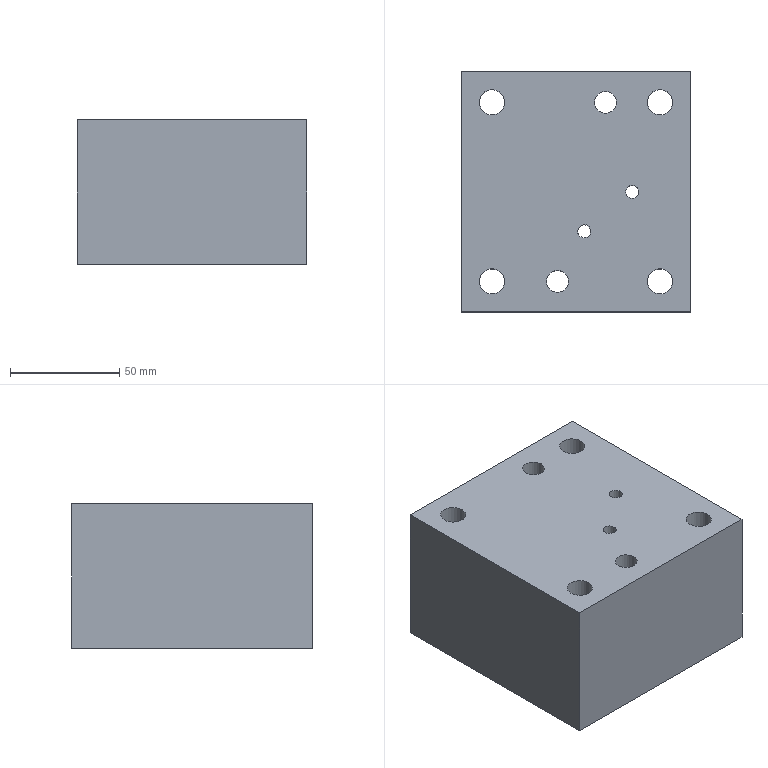Part | NX | features solid 2 | 1 solid | 32 faces | box 105 x 110 x 66.13 mm | volume 695141 mm3 | cylinder 16 | plane 12 | cone 4 | commonest cylinder face diameters 11.507 x4 18.008 x4 6 x2 8.5 x2 10 x2 12.505 x2
STEP:
#1=CARTESIAN_POINT('',(751.736,37.878,115.));
#2=VERTEX_POINT('',#1);
#3=CARTESIAN_POINT('',(751.736,28.874,115.));
#4=DIRECTION('',(0.000000053,-0.000000517,1.));
#5=DIRECTION('',(0.,1.,0.000000517));
#6=AXIS2_PLACEMENT_3D('',#3,#4,#5);
#7=CIRCLE('',#6,9.004);
#8=EDGE_CURVE('',#2,#2,#7,.T.);
#9=ORIENTED_EDGE('',*,*,#8,.T.);
#10=EDGE_LOOP('',(#9));
#11=FACE_BOUND('',#10,.T.);
#12=CARTESIAN_POINT('',(674.736,37.878,115.));
#13=VERTEX_POINT('',#12);
#14=CARTESIAN_POINT('',(674.736,28.874,115.));
#15=DIRECTION('',(0.000000053,-0.000000517,1.));
#16=DIRECTION('',(0.,1.,0.000000517));
#17=AXIS2_PLACEMENT_3D('',#14,#15,#16);
#18=CIRCLE('',#17,9.004);
#19=EDGE_CURVE('',#13,#13,#18,.T.);
#20=ORIENTED_EDGE('',*,*,#19,.T.);
#21=EDGE_LOOP('',(#20));
#22=FACE_BOUND('',#21,.T.);
#23=CARTESIAN_POINT('',(660.736,124.874,115.));
#24=VERTEX_POINT('',#23);
#25=CARTESIAN_POINT('',(660.736,14.874,115.));
#26=VERTEX_POINT('',#25);
#27=CARTESIAN_POINT('',(660.736,69.874,115.));
#28=DIRECTION('',(0.,1.,0.000000517));
#29=VECTOR('',#28,1000.);
#30=LINE('',#27,#29);
#31=EDGE_CURVE('',#24,#26,#30,.F.);
#32=ORIENTED_EDGE('',*,*,#31,.F.);
#33=CARTESIAN_POINT('',(765.736,124.874,115.));
#34=VERTEX_POINT('',#33);
#35=CARTESIAN_POINT('',(713.236,124.874,115.));
#36=DIRECTION('',(1.,0.,-0.000000053));
#37=VECTOR('',#36,1000.);
#38=LINE('',#35,#37);
#39=EDGE_CURVE('',#34,#24,#38,.F.);
#40=ORIENTED_EDGE('',*,*,#39,.F.);
#41=CARTESIAN_POINT('',(765.736,14.874,115.));
#42=VERTEX_POINT('',#41);
#43=CARTESIAN_POINT('',(765.736,69.874,115.));
#44=DIRECTION('',(0.,-1.,-0.000000517));
#45=VECTOR('',#44,1000.);
#46=LINE('',#43,#45);
#47=EDGE_CURVE('',#42,#34,#46,.F.);
#48=ORIENTED_EDGE('',*,*,#47,.F.);
#49=CARTESIAN_POINT('',(713.236,14.874,115.));
#50=DIRECTION('',(-1.,0.,0.000000053));
#51=VECTOR('',#50,1000.);
#52=LINE('',#49,#51);
#53=EDGE_CURVE('',#26,#42,#52,.F.);
#54=ORIENTED_EDGE('',*,*,#53,.F.);
#55=EDGE_LOOP('',(#32,#40,#48,#54));
#56=FACE_BOUND('',#55,.T.);
#57=CARTESIAN_POINT('',(751.736,119.878,115.));
#58=VERTEX_POINT('',#57);
#59=CARTESIAN_POINT('',(751.736,110.874,115.));
#60=DIRECTION('',(0.000000053,-0.000000517,1.));
#61=DIRECTION('',(0.,1.,0.000000517));
#62=AXIS2_PLACEMENT_3D('',#59,#60,#61);
#63=CIRCLE('',#62,9.004);
#64=EDGE_CURVE('',#58,#58,#63,.T.);
#65=ORIENTED_EDGE('',*,*,#64,.T.);
#66=EDGE_LOOP('',(#65));
#67=FACE_BOUND('',#66,.T.);
#68=CARTESIAN_POINT('',(674.736,119.878,115.));
#69=VERTEX_POINT('',#68);
#70=CARTESIAN_POINT('',(674.736,110.874,115.));
#71=DIRECTION('',(0.000000053,-0.000000517,1.));
#72=DIRECTION('',(0.,1.,0.000000517));
#73=AXIS2_PLACEMENT_3D('',#70,#71,#72);
#74=CIRCLE('',#73,9.004);
#75=EDGE_CURVE('',#69,#69,#74,.T.);
#76=ORIENTED_EDGE('',*,*,#75,.T.);
#77=EDGE_LOOP('',(#76));
#78=FACE_BOUND('',#77,.T.);
#79=CARTESIAN_POINT('',(726.736,117.126,115.));
#80=VERTEX_POINT('',#79);
#81=CARTESIAN_POINT('',(726.736,110.874,115.));
#82=DIRECTION('',(0.000000053,-0.000000517,1.));
#83=DIRECTION('',(0.,1.,0.000000517));
#84=AXIS2_PLACEMENT_3D('',#81,#82,#83);
#85=CIRCLE('',#84,6.253);
#86=EDGE_CURVE('',#80,#80,#85,.F.);
#87=ORIENTED_EDGE('',*,*,#86,.F.);
#88=EDGE_LOOP('',(#87));
#89=FACE_BOUND('',#88,.T.);
#90=CARTESIAN_POINT('',(704.736,35.126,115.));
#91=VERTEX_POINT('',#90);
#92=CARTESIAN_POINT('',(704.736,28.874,115.));
#93=DIRECTION('',(0.000000053,-0.000000517,1.));
#94=DIRECTION('',(0.,1.,0.000000517));
#95=AXIS2_PLACEMENT_3D('',#92,#93,#94);
#96=CIRCLE('',#95,6.253);
#97=EDGE_CURVE('',#91,#91,#96,.F.);
#98=ORIENTED_EDGE('',*,*,#97,.F.);
#99=EDGE_LOOP('',(#98));
#100=FACE_BOUND('',#99,.T.);
#101=CARTESIAN_POINT('',(729.986,79.874,115.));
#102=VERTEX_POINT('',#101);
#103=CARTESIAN_POINT('',(729.986,84.874,115.));
#104=DIRECTION('',(0.000000053,-0.000000517,1.));
#105=DIRECTION('',(0.,-1.,-0.000000517));
#106=AXIS2_PLACEMENT_3D('',#103,#104,#105);
#107=CIRCLE('',#106,5.);
#108=EDGE_CURVE('',#102,#102,#107,.T.);
#109=ORIENTED_EDGE('',*,*,#108,.T.);
#110=EDGE_LOOP('',(#109));
#111=FACE_BOUND('',#110,.T.);
#112=CARTESIAN_POINT('',(729.986,49.874,115.));
#113=VERTEX_POINT('',#112);
#114=CARTESIAN_POINT('',(729.986,54.874,115.));
#115=DIRECTION('',(0.000000053,-0.000000517,1.));
#116=DIRECTION('',(0.,-1.,-0.000000517));
#117=AXIS2_PLACEMENT_3D('',#114,#115,#116);
#118=CIRCLE('',#117,5.);
#119=EDGE_CURVE('',#113,#113,#118,.T.);
#120=ORIENTED_EDGE('',*,*,#119,.T.);
#121=EDGE_LOOP('',(#120));
#122=FACE_BOUND('',#121,.T.);
#123=CARTESIAN_POINT('',(716.986,48.874,115.));
#124=VERTEX_POINT('',#123);
#125=CARTESIAN_POINT('',(716.986,51.874,115.));
#126=DIRECTION('',(0.000000053,-0.000000517,1.));
#127=DIRECTION('',(0.,-1.,-0.000000517));
#128=AXIS2_PLACEMENT_3D('',#125,#126,#127);
#129=CIRCLE('',#128,3.);
#130=EDGE_CURVE('',#124,#124,#129,.F.);
#131=ORIENTED_EDGE('',*,*,#130,.F.);
#132=EDGE_LOOP('',(#131));
#133=FACE_BOUND('',#132,.T.);
#134=CARTESIAN_POINT('',(738.986,66.874,115.));
#135=VERTEX_POINT('',#134);
#136=CARTESIAN_POINT('',(738.986,69.874,115.));
#137=DIRECTION('',(0.000000053,-0.000000517,1.));
#138=DIRECTION('',(0.,-1.,-0.000000517));
#139=AXIS2_PLACEMENT_3D('',#136,#137,#138);
#140=CIRCLE('',#139,3.);
#141=EDGE_CURVE('',#135,#135,#140,.T.);
#142=ORIENTED_EDGE('',*,*,#141,.T.);
#143=EDGE_LOOP('',(#142));
#144=FACE_BOUND('',#143,.T.);
#145=CARTESIAN_POINT('',(735.986,94.874,115.));
#146=DIRECTION('',(0.000000053,-0.000000517,1.));
#147=DIRECTION('',(0.,1.,0.000000517));
#148=AXIS2_PLACEMENT_3D('',#145,#146,#147);
#149=PLANE('',#148);
#150=ADVANCED_FACE('',(#11,#22,#56,#67,#78,#89,#100,#111,#122,#133,#144),#149,.F.);
#151=CARTESIAN_POINT('',(660.736,124.874,181.13));
#152=VERTEX_POINT('',#151);
#153=CARTESIAN_POINT('',(765.736,124.874,181.13));
#154=VERTEX_POINT('',#153);
#155=CARTESIAN_POINT('',(713.236,124.874,181.13));
#156=DIRECTION('',(1.,0.,0.));
#157=VECTOR('',#156,1000.);
#158=LINE('',#155,#157);
#159=EDGE_CURVE('',#152,#154,#158,.T.);
#160=ORIENTED_EDGE('',*,*,#159,.F.);
#161=CARTESIAN_POINT('',(660.736,14.874,181.13));
#162=VERTEX_POINT('',#161);
#163=CARTESIAN_POINT('',(660.736,69.874,181.13));
#164=DIRECTION('',(0.,1.,0.));
#165=VECTOR('',#164,1000.);
#166=LINE('',#163,#165);
#167=EDGE_CURVE('',#162,#152,#166,.T.);
#168=ORIENTED_EDGE('',*,*,#167,.F.);
#169=CARTESIAN_POINT('',(765.736,14.874,181.13));
#170=VERTEX_POINT('',#169);
#171=CARTESIAN_POINT('',(713.236,14.874,181.13));
#172=DIRECTION('',(-1.,0.,0.));
#173=VECTOR('',#172,1000.);
#174=LINE('',#171,#173);
#175=EDGE_CURVE('',#170,#162,#174,.T.);
#176=ORIENTED_EDGE('',*,*,#175,.F.);
#177=CARTESIAN_POINT('',(765.736,69.874,181.13));
#178=DIRECTION('',(0.,-1.,0.));
#179=VECTOR('',#178,1000.);
#180=LINE('',#177,#179);
#181=EDGE_CURVE('',#154,#170,#180,.T.);
#182=ORIENTED_EDGE('',*,*,#181,.F.);
#183=EDGE_LOOP('',(#160,#168,#176,#182));
#184=FACE_BOUND('',#183,.T.);
#185=CARTESIAN_POINT('',(745.983,110.874,181.13));
#186=VERTEX_POINT('',#185);
#187=CARTESIAN_POINT('',(751.736,110.874,181.13));
#188=DIRECTION('',(0.,0.,1.));
#189=DIRECTION('',(-1.,0.,0.));
#190=AXIS2_PLACEMENT_3D('',#187,#188,#189);
#191=CIRCLE('',#190,5.753);
#192=EDGE_CURVE('',#186,#186,#191,.T.);
#193=ORIENTED_EDGE('',*,*,#192,.F.);
#194=EDGE_LOOP('',(#193));
#195=FACE_BOUND('',#194,.T.);
#196=CARTESIAN_POINT('',(668.983,28.874,181.13));
#197=VERTEX_POINT('',#196);
#198=CARTESIAN_POINT('',(674.736,28.874,181.13));
#199=DIRECTION('',(0.,0.,1.));
#200=DIRECTION('',(-1.,0.,0.));
#201=AXIS2_PLACEMENT_3D('',#198,#199,#200);
#202=CIRCLE('',#201,5.753);
#203=EDGE_CURVE('',#197,#197,#202,.T.);
#204=ORIENTED_EDGE('',*,*,#203,.F.);
#205=EDGE_LOOP('',(#204));
#206=FACE_BOUND('',#205,.T.);
#207=CARTESIAN_POINT('',(668.983,110.874,181.13));
#208=VERTEX_POINT('',#207);
#209=CARTESIAN_POINT('',(674.736,110.874,181.13));
#210=DIRECTION('',(0.,0.,1.));
#211=DIRECTION('',(-1.,0.,0.));
#212=AXIS2_PLACEMENT_3D('',#209,#210,#211);
#213=CIRCLE('',#212,5.753);
#214=EDGE_CURVE('',#208,#208,#213,.T.);
#215=ORIENTED_EDGE('',*,*,#214,.F.);
#216=EDGE_LOOP('',(#215));
#217=FACE_BOUND('',#216,.T.);
#218=CARTESIAN_POINT('',(745.983,28.874,181.13));
#219=VERTEX_POINT('',#218);
#220=CARTESIAN_POINT('',(751.736,28.874,181.13));
#221=DIRECTION('',(0.,0.,1.));
#222=DIRECTION('',(-1.,0.,0.));
#223=AXIS2_PLACEMENT_3D('',#220,#221,#222);
#224=CIRCLE('',#223,5.753);
#225=EDGE_CURVE('',#219,#219,#224,.T.);
#226=ORIENTED_EDGE('',*,*,#225,.F.);
#227=EDGE_LOOP('',(#226));
#228=FACE_BOUND('',#227,.T.);
#229=CARTESIAN_POINT('',(721.736,110.874,181.13));
#230=VERTEX_POINT('',#229);
#231=CARTESIAN_POINT('',(726.736,110.874,181.13));
#232=DIRECTION('',(0.,0.,1.));
#233=DIRECTION('',(-1.,0.,0.));
#234=AXIS2_PLACEMENT_3D('',#231,#232,#233);
#235=CIRCLE('',#234,5.);
#236=EDGE_CURVE('',#230,#230,#235,.T.);
#237=ORIENTED_EDGE('',*,*,#236,.F.);
#238=EDGE_LOOP('',(#237));
#239=FACE_BOUND('',#238,.T.);
#240=CARTESIAN_POINT('',(699.736,28.874,181.13));
#241=VERTEX_POINT('',#240);
#242=CARTESIAN_POINT('',(704.736,28.874,181.13));
#243=DIRECTION('',(0.,0.,1.));
#244=DIRECTION('',(-1.,0.,0.));
#245=AXIS2_PLACEMENT_3D('',#242,#243,#244);
#246=CIRCLE('',#245,5.);
#247=EDGE_CURVE('',#241,#241,#246,.T.);
#248=ORIENTED_EDGE('',*,*,#247,.F.);
#249=EDGE_LOOP('',(#248));
#250=FACE_BOUND('',#249,.T.);
#251=CARTESIAN_POINT('',(719.986,51.874,181.13));
#252=VERTEX_POINT('',#251);
#253=CARTESIAN_POINT('',(716.986,51.874,181.13));
#254=DIRECTION('',(0.,0.,1.));
#255=DIRECTION('',(1.,0.,0.));
#256=AXIS2_PLACEMENT_3D('',#253,#254,#255);
#257=CIRCLE('',#256,3.);
#258=EDGE_CURVE('',#252,#252,#257,.T.);
#259=ORIENTED_EDGE('',*,*,#258,.F.);
#260=EDGE_LOOP('',(#259));
#261=FACE_BOUND('',#260,.T.);
#262=CARTESIAN_POINT('',(741.986,69.874,181.13));
#263=VERTEX_POINT('',#262);
#264=CARTESIAN_POINT('',(738.986,69.874,181.13));
#265=DIRECTION('',(0.,0.,1.));
#266=DIRECTION('',(1.,0.,0.));
#267=AXIS2_PLACEMENT_3D('',#264,#265,#266);
#268=CIRCLE('',#267,3.);
#269=EDGE_CURVE('',#263,#263,#268,.F.);
#270=ORIENTED_EDGE('',*,*,#269,.T.);
#271=EDGE_LOOP('',(#270));
#272=FACE_BOUND('',#271,.T.);
#273=CARTESIAN_POINT('',(713.236,69.874,181.13));
#274=DIRECTION('',(0.,0.,1.));
#275=DIRECTION('',(-1.,0.,0.));
#276=AXIS2_PLACEMENT_3D('',#273,#274,#275);
#277=PLANE('',#276);
#278=ADVANCED_FACE('',(#184,#195,#206,#217,#228,#239,#250,#261,#272),#277,.T.);
#279=CARTESIAN_POINT('',(660.736,124.874,156.13));
#280=DIRECTION('',(0.,0.,1.));
#281=VECTOR('',#280,1000.);
#282=LINE('',#279,#281);
#283=EDGE_CURVE('',#24,#152,#282,.T.);
#284=ORIENTED_EDGE('',*,*,#283,.T.);
#285=ORIENTED_EDGE('',*,*,#159,.T.);
#286=CARTESIAN_POINT('',(765.736,124.874,156.13));
#287=DIRECTION('',(0.,0.,1.));
#288=VECTOR('',#287,1000.);
#289=LINE('',#286,#288);
#290=EDGE_CURVE('',#34,#154,#289,.T.);
#291=ORIENTED_EDGE('',*,*,#290,.F.);
#292=ORIENTED_EDGE('',*,*,#39,.T.);
#293=EDGE_LOOP('',(#284,#285,#291,#292));
#294=FACE_BOUND('',#293,.T.);
#295=CARTESIAN_POINT('',(713.236,124.874,156.13));
#296=DIRECTION('',(0.,1.,0.));
#297=DIRECTION('',(0.,0.,-1.));
#298=AXIS2_PLACEMENT_3D('',#295,#296,#297);
#299=PLANE('',#298);
#300=ADVANCED_FACE('',(#294),#299,.T.);
#301=ORIENTED_EDGE('',*,*,#290,.T.);
#302=ORIENTED_EDGE('',*,*,#181,.T.);
#303=CARTESIAN_POINT('',(765.736,14.874,156.13));
#304=DIRECTION('',(0.,0.,1.));
#305=VECTOR('',#304,1000.);
#306=LINE('',#303,#305);
#307=EDGE_CURVE('',#42,#170,#306,.T.);
#308=ORIENTED_EDGE('',*,*,#307,.F.);
#309=ORIENTED_EDGE('',*,*,#47,.T.);
#310=EDGE_LOOP('',(#301,#302,#308,#309));
#311=FACE_BOUND('',#310,.T.);
#312=CARTESIAN_POINT('',(765.736,69.874,156.13));
#313=DIRECTION('',(1.,0.,0.));
#314=DIRECTION('',(0.,0.,1.));
#315=AXIS2_PLACEMENT_3D('',#312,#313,#314);
#316=PLANE('',#315);
#317=ADVANCED_FACE('',(#311),#316,.T.);
#318=ORIENTED_EDGE('',*,*,#307,.T.);
#319=ORIENTED_EDGE('',*,*,#175,.T.);
#320=CARTESIAN_POINT('',(660.736,14.874,156.13));
#321=DIRECTION('',(0.,0.,1.));
#322=VECTOR('',#321,1000.);
#323=LINE('',#320,#322);
#324=EDGE_CURVE('',#26,#162,#323,.T.);
#325=ORIENTED_EDGE('',*,*,#324,.F.);
#326=ORIENTED_EDGE('',*,*,#53,.T.);
#327=EDGE_LOOP('',(#318,#319,#325,#326));
#328=FACE_BOUND('',#327,.T.);
#329=CARTESIAN_POINT('',(713.236,14.874,156.13));
#330=DIRECTION('',(0.,-1.,0.));
#331=DIRECTION('',(0.,0.,1.));
#332=AXIS2_PLACEMENT_3D('',#329,#330,#331);
#333=PLANE('',#332);
#334=ADVANCED_FACE('',(#328),#333,.T.);
#335=ORIENTED_EDGE('',*,*,#31,.T.);
#336=ORIENTED_EDGE('',*,*,#324,.T.);
#337=ORIENTED_EDGE('',*,*,#167,.T.);
#338=ORIENTED_EDGE('',*,*,#283,.F.);
#339=EDGE_LOOP('',(#335,#336,#337,#338));
#340=FACE_BOUND('',#339,.T.);
#341=CARTESIAN_POINT('',(660.736,69.874,156.13));
#342=DIRECTION('',(-1.,0.,0.));
#343=DIRECTION('',(0.,0.,-1.));
#344=AXIS2_PLACEMENT_3D('',#341,#342,#343);
#345=PLANE('',#344);
#346=ADVANCED_FACE('',(#340),#345,.T.);
#347=ORIENTED_EDGE('',*,*,#192,.T.);
#348=EDGE_LOOP('',(#347));
#349=FACE_BOUND('',#348,.T.);
#350=CARTESIAN_POINT('',(745.983,110.874,149.13));
#351=VERTEX_POINT('',#350);
#352=CARTESIAN_POINT('',(751.736,110.874,149.13));
#353=DIRECTION('',(0.,0.,1.));
#354=DIRECTION('',(-1.,0.,0.));
#355=AXIS2_PLACEMENT_3D('',#352,#353,#354);
#356=CIRCLE('',#355,5.753);
#357=EDGE_CURVE('',#351,#351,#356,.T.);
#358=ORIENTED_EDGE('',*,*,#357,.F.);
#359=EDGE_LOOP('',(#358));
#360=FACE_BOUND('',#359,.T.);
#361=CARTESIAN_POINT('',(751.736,110.874,153.13));
#362=DIRECTION('',(0.,0.,1.));
#363=DIRECTION('',(-1.,0.,0.));
#364=AXIS2_PLACEMENT_3D('',#361,#362,#363);
#365=CYLINDRICAL_SURFACE('',#364,5.753);
#366=ADVANCED_FACE('',(#349,#360),#365,.F.);
#367=ORIENTED_EDGE('',*,*,#357,.T.);
#368=EDGE_LOOP('',(#367));
#369=FACE_BOUND('',#368,.T.);
#370=CARTESIAN_POINT('',(742.732,110.874,149.13));
#371=VERTEX_POINT('',#370);
#372=CARTESIAN_POINT('',(751.736,110.874,149.13));
#373=DIRECTION('',(0.,0.,-1.));
#374=DIRECTION('',(-1.,0.,0.));
#375=AXIS2_PLACEMENT_3D('',#372,#373,#374);
#376=CIRCLE('',#375,9.004);
#377=EDGE_CURVE('',#371,#371,#376,.F.);
#378=ORIENTED_EDGE('',*,*,#377,.F.);
#379=EDGE_LOOP('',(#378));
#380=FACE_BOUND('',#379,.T.);
#381=CARTESIAN_POINT('',(751.736,110.874,149.13));
#382=DIRECTION('',(0.,0.,1.));
#383=DIRECTION('',(-1.,0.,0.));
#384=AXIS2_PLACEMENT_3D('',#381,#382,#383);
#385=PLANE('',#384);
#386=ADVANCED_FACE('',(#369,#380),#385,.F.);
#387=ORIENTED_EDGE('',*,*,#377,.T.);
#388=EDGE_LOOP('',(#387));
#389=FACE_BOUND('',#388,.T.);
#390=ORIENTED_EDGE('',*,*,#64,.F.);
#391=EDGE_LOOP('',(#390));
#392=FACE_BOUND('',#391,.T.);
#393=CARTESIAN_POINT('',(751.736,110.874,156.13));
#394=DIRECTION('',(0.,0.,1.));
#395=DIRECTION('',(-1.,0.,0.));
#396=AXIS2_PLACEMENT_3D('',#393,#394,#395);
#397=CYLINDRICAL_SURFACE('',#396,9.004);
#398=ADVANCED_FACE('',(#389,#392),#397,.F.);
#399=ORIENTED_EDGE('',*,*,#203,.T.);
#400=EDGE_LOOP('',(#399));
#401=FACE_BOUND('',#400,.T.);
#402=CARTESIAN_POINT('',(668.983,28.874,149.13));
#403=VERTEX_POINT('',#402);
#404=CARTESIAN_POINT('',(674.736,28.874,149.13));
#405=DIRECTION('',(0.,0.,1.));
#406=DIRECTION('',(-1.,0.,0.));
#407=AXIS2_PLACEMENT_3D('',#404,#405,#406);
#408=CIRCLE('',#407,5.753);
#409=EDGE_CURVE('',#403,#403,#408,.T.);
#410=ORIENTED_EDGE('',*,*,#409,.F.);
#411=EDGE_LOOP('',(#410));
#412=FACE_BOUND('',#411,.T.);
#413=CARTESIAN_POINT('',(674.736,28.874,153.13));
#414=DIRECTION('',(0.,0.,1.));
#415=DIRECTION('',(-1.,0.,0.));
#416=AXIS2_PLACEMENT_3D('',#413,#414,#415);
#417=CYLINDRICAL_SURFACE('',#416,5.753);
#418=ADVANCED_FACE('',(#401,#412),#417,.F.);
#419=ORIENTED_EDGE('',*,*,#409,.T.);
#420=EDGE_LOOP('',(#419));
#421=FACE_BOUND('',#420,.T.);
#422=CARTESIAN_POINT('',(665.732,28.874,149.13));
#423=VERTEX_POINT('',#422);
#424=CARTESIAN_POINT('',(674.736,28.874,149.13));
#425=DIRECTION('',(0.,0.,-1.));
#426=DIRECTION('',(-1.,0.,0.));
#427=AXIS2_PLACEMENT_3D('',#424,#425,#426);
#428=CIRCLE('',#427,9.004);
#429=EDGE_CURVE('',#423,#423,#428,.F.);
#430=ORIENTED_EDGE('',*,*,#429,.F.);
#431=EDGE_LOOP('',(#430));
#432=FACE_BOUND('',#431,.T.);
#433=CARTESIAN_POINT('',(674.736,28.874,149.13));
#434=DIRECTION('',(0.,0.,1.));
#435=DIRECTION('',(-1.,0.,0.));
#436=AXIS2_PLACEMENT_3D('',#433,#434,#435);
#437=PLANE('',#436);
#438=ADVANCED_FACE('',(#421,#432),#437,.F.);
#439=ORIENTED_EDGE('',*,*,#429,.T.);
#440=EDGE_LOOP('',(#439));
#441=FACE_BOUND('',#440,.T.);
#442=ORIENTED_EDGE('',*,*,#19,.F.);
#443=EDGE_LOOP('',(#442));
#444=FACE_BOUND('',#443,.T.);
#445=CARTESIAN_POINT('',(674.736,28.874,156.13));
#446=DIRECTION('',(0.,0.,1.));
#447=DIRECTION('',(-1.,0.,0.));
#448=AXIS2_PLACEMENT_3D('',#445,#446,#447);
#449=CYLINDRICAL_SURFACE('',#448,9.004);
#450=ADVANCED_FACE('',(#441,#444),#449,.F.);
#451=ORIENTED_EDGE('',*,*,#214,.T.);
#452=EDGE_LOOP('',(#451));
#453=FACE_BOUND('',#452,.T.);
#454=CARTESIAN_POINT('',(668.983,110.874,149.13));
#455=VERTEX_POINT('',#454);
#456=CARTESIAN_POINT('',(674.736,110.874,149.13));
#457=DIRECTION('',(0.,0.,1.));
#458=DIRECTION('',(-1.,0.,0.));
#459=AXIS2_PLACEMENT_3D('',#456,#457,#458);
#460=CIRCLE('',#459,5.753);
#461=EDGE_CURVE('',#455,#455,#460,.T.);
#462=ORIENTED_EDGE('',*,*,#461,.F.);
#463=EDGE_LOOP('',(#462));
#464=FACE_BOUND('',#463,.T.);
#465=CARTESIAN_POINT('',(674.736,110.874,153.13));
#466=DIRECTION('',(0.,0.,1.));
#467=DIRECTION('',(-1.,0.,0.));
#468=AXIS2_PLACEMENT_3D('',#465,#466,#467);
#469=CYLINDRICAL_SURFACE('',#468,5.753);
#470=ADVANCED_FACE('',(#453,#464),#469,.F.);
#471=ORIENTED_EDGE('',*,*,#461,.T.);
#472=EDGE_LOOP('',(#471));
#473=FACE_BOUND('',#472,.T.);
#474=CARTESIAN_POINT('',(665.732,110.874,149.13));
#475=VERTEX_POINT('',#474);
#476=CARTESIAN_POINT('',(674.736,110.874,149.13));
#477=DIRECTION('',(0.,0.,-1.));
#478=DIRECTION('',(-1.,0.,0.));
#479=AXIS2_PLACEMENT_3D('',#476,#477,#478);
#480=CIRCLE('',#479,9.004);
#481=EDGE_CURVE('',#475,#475,#480,.F.);
#482=ORIENTED_EDGE('',*,*,#481,.F.);
#483=EDGE_LOOP('',(#482));
#484=FACE_BOUND('',#483,.T.);
#485=CARTESIAN_POINT('',(674.736,110.874,149.13));
#486=DIRECTION('',(0.,0.,1.));
#487=DIRECTION('',(-1.,0.,0.));
#488=AXIS2_PLACEMENT_3D('',#485,#486,#487);
#489=PLANE('',#488);
#490=ADVANCED_FACE('',(#473,#484),#489,.F.);
#491=ORIENTED_EDGE('',*,*,#481,.T.);
#492=EDGE_LOOP('',(#491));
#493=FACE_BOUND('',#492,.T.);
#494=ORIENTED_EDGE('',*,*,#75,.F.);
#495=EDGE_LOOP('',(#494));
#496=FACE_BOUND('',#495,.T.);
#497=CARTESIAN_POINT('',(674.736,110.874,156.13));
#498=DIRECTION('',(0.,0.,1.));
#499=DIRECTION('',(-1.,0.,0.));
#500=AXIS2_PLACEMENT_3D('',#497,#498,#499);
#501=CYLINDRICAL_SURFACE('',#500,9.004);
#502=ADVANCED_FACE('',(#493,#496),#501,.F.);
#503=ORIENTED_EDGE('',*,*,#225,.T.);
#504=EDGE_LOOP('',(#503));
#505=FACE_BOUND('',#504,.T.);
#506=CARTESIAN_POINT('',(745.983,28.874,149.13));
#507=VERTEX_POINT('',#506);
#508=CARTESIAN_POINT('',(751.736,28.874,149.13));
#509=DIRECTION('',(0.,0.,1.));
#510=DIRECTION('',(-1.,0.,0.));
#511=AXIS2_PLACEMENT_3D('',#508,#509,#510);
#512=CIRCLE('',#511,5.753);
#513=EDGE_CURVE('',#507,#507,#512,.T.);
#514=ORIENTED_EDGE('',*,*,#513,.F.);
#515=EDGE_LOOP('',(#514));
#516=FACE_BOUND('',#515,.T.);
#517=CARTESIAN_POINT('',(751.736,28.874,153.13));
#518=DIRECTION('',(0.,0.,1.));
#519=DIRECTION('',(-1.,0.,0.));
#520=AXIS2_PLACEMENT_3D('',#517,#518,#519);
#521=CYLINDRICAL_SURFACE('',#520,5.753);
#522=ADVANCED_FACE('',(#505,#516),#521,.F.);
#523=ORIENTED_EDGE('',*,*,#513,.T.);
#524=EDGE_LOOP('',(#523));
#525=FACE_BOUND('',#524,.T.);
#526=CARTESIAN_POINT('',(742.732,28.874,149.13));
#527=VERTEX_POINT('',#526);
#528=CARTESIAN_POINT('',(751.736,28.874,149.13));
#529=DIRECTION('',(0.,0.,-1.));
#530=DIRECTION('',(-1.,0.,0.));
#531=AXIS2_PLACEMENT_3D('',#528,#529,#530);
#532=CIRCLE('',#531,9.004);
#533=EDGE_CURVE('',#527,#527,#532,.F.);
#534=ORIENTED_EDGE('',*,*,#533,.F.);
#535=EDGE_LOOP('',(#534));
#536=FACE_BOUND('',#535,.T.);
#537=CARTESIAN_POINT('',(751.736,28.874,149.13));
#538=DIRECTION('',(0.,0.,1.));
#539=DIRECTION('',(-1.,0.,0.));
#540=AXIS2_PLACEMENT_3D('',#537,#538,#539);
#541=PLANE('',#540);
#542=ADVANCED_FACE('',(#525,#536),#541,.F.);
#543=ORIENTED_EDGE('',*,*,#533,.T.);
#544=EDGE_LOOP('',(#543));
#545=FACE_BOUND('',#544,.T.);
#546=ORIENTED_EDGE('',*,*,#8,.F.);
#547=EDGE_LOOP('',(#546));
#548=FACE_BOUND('',#547,.T.);
#549=CARTESIAN_POINT('',(751.736,28.874,156.13));
#550=DIRECTION('',(0.,0.,1.));
#551=DIRECTION('',(-1.,0.,0.));
#552=AXIS2_PLACEMENT_3D('',#549,#550,#551);
#553=CYLINDRICAL_SURFACE('',#552,9.004);
#554=ADVANCED_FACE('',(#545,#548),#553,.F.);
#555=ORIENTED_EDGE('',*,*,#236,.T.);
#556=EDGE_LOOP('',(#555));
#557=FACE_BOUND('',#556,.T.);
#558=CARTESIAN_POINT('',(721.736,110.874,148.13));
#559=VERTEX_POINT('',#558);
#560=CARTESIAN_POINT('',(726.736,110.874,148.13));
#561=DIRECTION('',(0.,0.,1.));
#562=DIRECTION('',(-1.,0.,0.));
#563=AXIS2_PLACEMENT_3D('',#560,#561,#562);
#564=CIRCLE('',#563,5.);
#565=EDGE_CURVE('',#559,#559,#564,.T.);
#566=ORIENTED_EDGE('',*,*,#565,.F.);
#567=EDGE_LOOP('',(#566));
#568=FACE_BOUND('',#567,.T.);
#569=CARTESIAN_POINT('',(726.736,110.874,153.13));
#570=DIRECTION('',(0.,0.,1.));
#571=DIRECTION('',(-1.,0.,0.));
#572=AXIS2_PLACEMENT_3D('',#569,#570,#571);
#573=CYLINDRICAL_SURFACE('',#572,5.);
#574=ADVANCED_FACE('',(#557,#568),#573,.F.);
#575=ORIENTED_EDGE('',*,*,#565,.T.);
#576=EDGE_LOOP('',(#575));
#577=FACE_BOUND('',#576,.T.);
#578=CARTESIAN_POINT('',(720.484,110.874,148.13));
#579=VERTEX_POINT('',#578);
#580=CARTESIAN_POINT('',(726.736,110.874,148.13));
#581=DIRECTION('',(0.,0.,-1.));
#582=DIRECTION('',(-1.,0.,0.));
#583=AXIS2_PLACEMENT_3D('',#580,#581,#582);
#584=CIRCLE('',#583,6.253);
#585=EDGE_CURVE('',#579,#579,#584,.F.);
#586=ORIENTED_EDGE('',*,*,#585,.F.);
#587=EDGE_LOOP('',(#586));
#588=FACE_BOUND('',#587,.T.);
#589=CARTESIAN_POINT('',(726.736,110.874,148.13));
#590=DIRECTION('',(0.,0.,1.));
#591=DIRECTION('',(-1.,0.,0.));
#592=AXIS2_PLACEMENT_3D('',#589,#590,#591);
#593=PLANE('',#592);
#594=ADVANCED_FACE('',(#577,#588),#593,.F.);
#595=ORIENTED_EDGE('',*,*,#86,.T.);
#596=EDGE_LOOP('',(#595));
#597=FACE_BOUND('',#596,.T.);
#598=ORIENTED_EDGE('',*,*,#585,.T.);
#599=EDGE_LOOP('',(#598));
#600=FACE_BOUND('',#599,.T.);
#601=CARTESIAN_POINT('',(726.736,110.874,153.13));
#602=DIRECTION('',(0.,0.,1.));
#603=DIRECTION('',(-1.,0.,0.));
#604=AXIS2_PLACEMENT_3D('',#601,#602,#603);
#605=CYLINDRICAL_SURFACE('',#604,6.253);
#606=ADVANCED_FACE('',(#597,#600),#605,.F.);
#607=ORIENTED_EDGE('',*,*,#247,.T.);
#608=EDGE_LOOP('',(#607));
#609=FACE_BOUND('',#608,.T.);
#610=CARTESIAN_POINT('',(699.736,28.874,148.13));
#611=VERTEX_POINT('',#610);
#612=CARTESIAN_POINT('',(704.736,28.874,148.13));
#613=DIRECTION('',(0.,0.,1.));
#614=DIRECTION('',(-1.,0.,0.));
#615=AXIS2_PLACEMENT_3D('',#612,#613,#614);
#616=CIRCLE('',#615,5.);
#617=EDGE_CURVE('',#611,#611,#616,.T.);
#618=ORIENTED_EDGE('',*,*,#617,.F.);
#619=EDGE_LOOP('',(#618));
#620=FACE_BOUND('',#619,.T.);
#621=CARTESIAN_POINT('',(704.736,28.874,153.13));
#622=DIRECTION('',(0.,0.,1.));
#623=DIRECTION('',(-1.,0.,0.));
#624=AXIS2_PLACEMENT_3D('',#621,#622,#623);
#625=CYLINDRICAL_SURFACE('',#624,5.);
#626=ADVANCED_FACE('',(#609,#620),#625,.F.);
#627=ORIENTED_EDGE('',*,*,#617,.T.);
#628=EDGE_LOOP('',(#627));
#629=FACE_BOUND('',#628,.T.);
#630=CARTESIAN_POINT('',(698.484,28.874,148.13));
#631=VERTEX_POINT('',#630);
#632=CARTESIAN_POINT('',(704.736,28.874,148.13));
#633=DIRECTION('',(0.,0.,-1.));
#634=DIRECTION('',(-1.,0.,0.));
#635=AXIS2_PLACEMENT_3D('',#632,#633,#634);
#636=CIRCLE('',#635,6.253);
#637=EDGE_CURVE('',#631,#631,#636,.F.);
#638=ORIENTED_EDGE('',*,*,#637,.F.);
#639=EDGE_LOOP('',(#638));
#640=FACE_BOUND('',#639,.T.);
#641=CARTESIAN_POINT('',(704.736,28.874,148.13));
#642=DIRECTION('',(0.,0.,1.));
#643=DIRECTION('',(-1.,0.,0.));
#644=AXIS2_PLACEMENT_3D('',#641,#642,#643);
#645=PLANE('',#644);
#646=ADVANCED_FACE('',(#629,#640),#645,.F.);
#647=ORIENTED_EDGE('',*,*,#97,.T.);
#648=EDGE_LOOP('',(#647));
#649=FACE_BOUND('',#648,.T.);
#650=ORIENTED_EDGE('',*,*,#637,.T.);
#651=EDGE_LOOP('',(#650));
#652=FACE_BOUND('',#651,.T.);
#653=CARTESIAN_POINT('',(704.736,28.874,153.13));
#654=DIRECTION('',(0.,0.,1.));
#655=DIRECTION('',(-1.,0.,0.));
#656=AXIS2_PLACEMENT_3D('',#653,#654,#655);
#657=CYLINDRICAL_SURFACE('',#656,6.253);
#658=ADVANCED_FACE('',(#649,#652),#657,.F.);
#659=CARTESIAN_POINT('',(729.986,80.624,145.));
#660=VERTEX_POINT('',#659);
#661=CARTESIAN_POINT('',(729.986,84.874,145.));
#662=DIRECTION('',(0.000000053,-0.000000517,1.));
#663=DIRECTION('',(0.,-1.,-0.000000517));
#664=AXIS2_PLACEMENT_3D('',#661,#662,#663);
#665=CIRCLE('',#664,4.25);
#666=EDGE_CURVE('',#660,#660,#665,.F.);
#667=ORIENTED_EDGE('',*,*,#666,.T.);
#668=EDGE_LOOP('',(#667));
#669=FACE_BOUND('',#668,.T.);
#670=CARTESIAN_POINT('',(729.986,84.874,147.553));
#671=VERTEX_POINT('',#670);
#672=VERTEX_LOOP('',#671);
#673=FACE_BOUND('',#672,.T.);
#674=CARTESIAN_POINT('',(729.986,84.874,145.));
#675=DIRECTION('',(-0.000000053,0.000000517,-1.));
#676=DIRECTION('',(0.,1.,0.000000517));
#677=AXIS2_PLACEMENT_3D('',#674,#675,#676);
#678=CONICAL_SURFACE('',#677,4.25,1.03);
#679=ADVANCED_FACE('',(#669,#673),#678,.F.);
#680=CARTESIAN_POINT('',(729.986,89.124,115.75));
#681=VERTEX_POINT('',#680);
#682=CARTESIAN_POINT('',(729.986,84.874,115.75));
#683=DIRECTION('',(-0.000000053,0.000000517,-1.));
#684=DIRECTION('',(0.,1.,0.000000517));
#685=AXIS2_PLACEMENT_3D('',#682,#683,#684);
#686=CIRCLE('',#685,4.25);
#687=EDGE_CURVE('',#681,#681,#686,.T.);
#688=ORIENTED_EDGE('',*,*,#687,.T.);
#689=EDGE_LOOP('',(#688));
#690=FACE_BOUND('',#689,.T.);
#691=ORIENTED_EDGE('',*,*,#666,.F.);
#692=EDGE_LOOP('',(#691));
#693=FACE_BOUND('',#692,.T.);
#694=CARTESIAN_POINT('',(729.986,84.874,115.));
#695=DIRECTION('',(0.000000053,-0.000000517,1.));
#696=DIRECTION('',(0.,-1.,-0.000000517));
#697=AXIS2_PLACEMENT_3D('',#694,#695,#696);
#698=CYLINDRICAL_SURFACE('',#697,4.25);
#699=ADVANCED_FACE('',(#690,#693),#698,.F.);
#700=ORIENTED_EDGE('',*,*,#687,.F.);
#701=EDGE_LOOP('',(#700));
#702=FACE_BOUND('',#701,.T.);
#703=ORIENTED_EDGE('',*,*,#108,.F.);
#704=EDGE_LOOP('',(#703));
#705=FACE_BOUND('',#704,.T.);
#706=CARTESIAN_POINT('',(729.986,84.874,115.));
#707=DIRECTION('',(-0.000000053,0.000000517,-1.));
#708=DIRECTION('',(0.,1.,0.000000517));
#709=AXIS2_PLACEMENT_3D('',#706,#707,#708);
#710=CONICAL_SURFACE('',#709,5.,0.7854);
#711=ADVANCED_FACE('',(#702,#705),#710,.F.);
#712=CARTESIAN_POINT('',(729.986,50.624,145.));
#713=VERTEX_POINT('',#712);
#714=CARTESIAN_POINT('',(729.986,54.874,145.));
#715=DIRECTION('',(0.000000053,-0.000000517,1.));
#716=DIRECTION('',(0.,-1.,-0.000000517));
#717=AXIS2_PLACEMENT_3D('',#714,#715,#716);
#718=CIRCLE('',#717,4.25);
#719=EDGE_CURVE('',#713,#713,#718,.F.);
#720=ORIENTED_EDGE('',*,*,#719,.T.);
#721=EDGE_LOOP('',(#720));
#722=FACE_BOUND('',#721,.T.);
#723=CARTESIAN_POINT('',(729.986,54.874,147.553));
#724=VERTEX_POINT('',#723);
#725=VERTEX_LOOP('',#724);
#726=FACE_BOUND('',#725,.T.);
#727=CARTESIAN_POINT('',(729.986,54.874,145.));
#728=DIRECTION('',(-0.000000053,0.000000517,-1.));
#729=DIRECTION('',(0.,1.,0.000000517));
#730=AXIS2_PLACEMENT_3D('',#727,#728,#729);
#731=CONICAL_SURFACE('',#730,4.25,1.03);
#732=ADVANCED_FACE('',(#722,#726),#731,.F.);
#733=CARTESIAN_POINT('',(729.986,59.124,115.75));
#734=VERTEX_POINT('',#733);
#735=CARTESIAN_POINT('',(729.986,54.874,115.75));
#736=DIRECTION('',(-0.000000053,0.000000517,-1.));
#737=DIRECTION('',(0.,1.,0.000000517));
#738=AXIS2_PLACEMENT_3D('',#735,#736,#737);
#739=CIRCLE('',#738,4.25);
#740=EDGE_CURVE('',#734,#734,#739,.T.);
#741=ORIENTED_EDGE('',*,*,#740,.T.);
#742=EDGE_LOOP('',(#741));
#743=FACE_BOUND('',#742,.T.);
#744=ORIENTED_EDGE('',*,*,#719,.F.);
#745=EDGE_LOOP('',(#744));
#746=FACE_BOUND('',#745,.T.);
#747=CARTESIAN_POINT('',(729.986,54.874,115.));
#748=DIRECTION('',(0.000000053,-0.000000517,1.));
#749=DIRECTION('',(0.,-1.,-0.000000517));
#750=AXIS2_PLACEMENT_3D('',#747,#748,#749);
#751=CYLINDRICAL_SURFACE('',#750,4.25);
#752=ADVANCED_FACE('',(#743,#746),#751,.F.);
#753=ORIENTED_EDGE('',*,*,#740,.F.);
#754=EDGE_LOOP('',(#753));
#755=FACE_BOUND('',#754,.T.);
#756=ORIENTED_EDGE('',*,*,#119,.F.);
#757=EDGE_LOOP('',(#756));
#758=FACE_BOUND('',#757,.T.);
#759=CARTESIAN_POINT('',(729.986,54.874,115.));
#760=DIRECTION('',(-0.000000053,0.000000517,-1.));
#761=DIRECTION('',(0.,1.,0.000000517));
#762=AXIS2_PLACEMENT_3D('',#759,#760,#761);
#763=CONICAL_SURFACE('',#762,5.,0.7854);
#764=ADVANCED_FACE('',(#755,#758),#763,.F.);
#765=ORIENTED_EDGE('',*,*,#130,.T.);
#766=EDGE_LOOP('',(#765));
#767=FACE_BOUND('',#766,.T.);
#768=ORIENTED_EDGE('',*,*,#258,.T.);
#769=EDGE_LOOP('',(#768));
#770=FACE_BOUND('',#769,.T.);
#771=CARTESIAN_POINT('',(716.986,51.874,-720.));
#772=DIRECTION('',(0.000000053,-0.000000517,1.));
#773=DIRECTION('',(0.,-1.,-0.000000517));
#774=AXIS2_PLACEMENT_3D('',#771,#772,#773);
#775=CYLINDRICAL_SURFACE('',#774,3.);
#776=ADVANCED_FACE('',(#767,#770),#775,.F.);
#777=ORIENTED_EDGE('',*,*,#141,.F.);
#778=EDGE_LOOP('',(#777));
#779=FACE_BOUND('',#778,.T.);
#780=ORIENTED_EDGE('',*,*,#269,.F.);
#781=EDGE_LOOP('',(#780));
#782=FACE_BOUND('',#781,.T.);
#783=CARTESIAN_POINT('',(738.986,69.874,-720.));
#784=DIRECTION('',(0.000000053,-0.000000517,1.));
#785=DIRECTION('',(0.,-1.,-0.000000517));
#786=AXIS2_PLACEMENT_3D('',#783,#784,#785);
#787=CYLINDRICAL_SURFACE('',#786,3.);
#788=ADVANCED_FACE('',(#779,#782),#787,.F.);
#789=CLOSED_SHELL('',(#150,#278,#300,#317,#334,#346,#366,#386,#398,#418,#438,#450,#470,#490,#502,#522,#542,#554,#574,#594,#606,#626,#646,#658,#679,#699,#711,#732,#752,#764,#776,#788));
#790=MANIFOLD_SOLID_BREP('',#789);
#791=(LENGTH_UNIT()NAMED_UNIT(*)SI_UNIT(.MILLI.,.METRE.));
#792=UNCERTAINTY_MEASURE_WITH_UNIT(LENGTH_MEASURE(0.00001),#791,'','');
#793=(NAMED_UNIT(*)PLANE_ANGLE_UNIT()SI_UNIT($,.RADIAN.));
#794=(NAMED_UNIT(*)SI_UNIT($,.STERADIAN.)SOLID_ANGLE_UNIT());
#795=(GEOMETRIC_REPRESENTATION_CONTEXT(3)GLOBAL_UNCERTAINTY_ASSIGNED_CONTEXT((#792))GLOBAL_UNIT_ASSIGNED_CONTEXT((#791,#793,#794))REPRESENTATION_CONTEXT('',''));
#796=ADVANCED_BREP_SHAPE_REPRESENTATION('',(#790),#795);